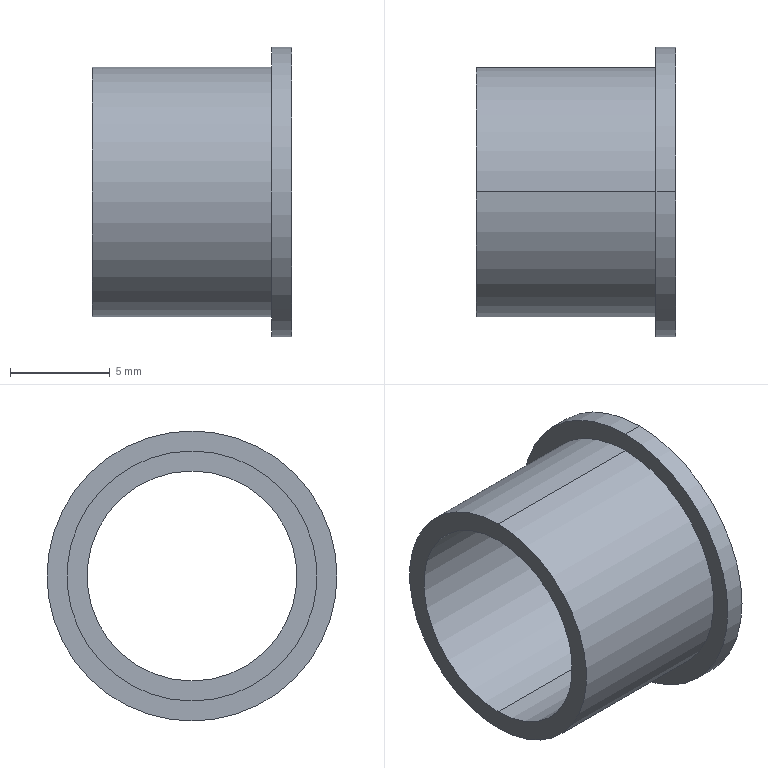Part | SolidWorks | features BaseBody 1 | 1 solid | 9 faces | box 10 x 14.5 x 14.5 mm | volume 403.695 mm3 | cylinder 6 | plane 3 | commonest cylinder face diameters 10.5 x2 12.5 x2 14.5 x2
STEP:
#1=CARTESIAN_POINT('',(6.037,-20.104,-31.5));
#2=VERTEX_POINT('',#1);
#3=CARTESIAN_POINT('',(6.037,-20.104,-46.));
#4=VERTEX_POINT('',#3);
#5=CARTESIAN_POINT('',(6.037,-20.104,-38.75));
#6=DIRECTION('',(-1.,0.,0.));
#7=DIRECTION('',(0.,0.,1.));
#8=AXIS2_PLACEMENT_3D('',#5,#6,#7);
#9=CIRCLE('',#8,7.25);
#10=EDGE_CURVE('',#2,#4,#9,.T.);
#11=ORIENTED_EDGE('',*,*,#10,.F.);
#12=CARTESIAN_POINT('',(7.037,-20.104,-31.5));
#13=VERTEX_POINT('',#12);
#14=CARTESIAN_POINT('',(6.037,-20.104,-31.5));
#15=DIRECTION('',(1.,0.,0.));
#16=VECTOR('',#15,1000.);
#17=LINE('',#14,#16);
#18=EDGE_CURVE('',#2,#13,#17,.T.);
#19=ORIENTED_EDGE('',*,*,#18,.T.);
#20=CARTESIAN_POINT('',(7.037,-20.104,-46.));
#21=VERTEX_POINT('',#20);
#22=CARTESIAN_POINT('',(7.037,-20.104,-38.75));
#23=DIRECTION('',(-1.,0.,0.));
#24=DIRECTION('',(0.,0.,1.));
#25=AXIS2_PLACEMENT_3D('',#22,#23,#24);
#26=CIRCLE('',#25,7.25);
#27=EDGE_CURVE('',#13,#21,#26,.T.);
#28=ORIENTED_EDGE('',*,*,#27,.T.);
#29=CARTESIAN_POINT('',(6.037,-20.104,-46.));
#30=DIRECTION('',(1.,0.,0.));
#31=VECTOR('',#30,1000.);
#32=LINE('',#29,#31);
#33=EDGE_CURVE('',#4,#21,#32,.T.);
#34=ORIENTED_EDGE('',*,*,#33,.F.);
#35=EDGE_LOOP('',(#11,#19,#28,#34));
#36=FACE_OUTER_BOUND('',#35,.T.);
#37=CARTESIAN_POINT('',(6.037,-20.104,-38.75));
#38=DIRECTION('',(1.,0.,0.));
#39=DIRECTION('',(0.,0.,-1.));
#40=AXIS2_PLACEMENT_3D('',#37,#38,#39);
#41=CYLINDRICAL_SURFACE('',#40,7.25);
#42=ADVANCED_FACE('',(#36),#41,.T.);
#43=CARTESIAN_POINT('',(-2.963,-20.104,-32.5));
#44=VERTEX_POINT('',#43);
#45=CARTESIAN_POINT('',(-2.963,-20.104,-45.));
#46=VERTEX_POINT('',#45);
#47=CARTESIAN_POINT('',(-2.963,-20.104,-38.75));
#48=DIRECTION('',(-1.,0.,0.));
#49=DIRECTION('',(0.,0.,1.));
#50=AXIS2_PLACEMENT_3D('',#47,#48,#49);
#51=CIRCLE('',#50,6.25);
#52=EDGE_CURVE('',#44,#46,#51,.T.);
#53=ORIENTED_EDGE('',*,*,#52,.F.);
#54=CARTESIAN_POINT('',(6.037,-20.104,-32.5));
#55=VERTEX_POINT('',#54);
#56=CARTESIAN_POINT('',(-2.963,-20.104,-32.5));
#57=DIRECTION('',(1.,0.,0.));
#58=VECTOR('',#57,1000.);
#59=LINE('',#56,#58);
#60=EDGE_CURVE('',#44,#55,#59,.T.);
#61=ORIENTED_EDGE('',*,*,#60,.T.);
#62=CARTESIAN_POINT('',(6.037,-20.104,-45.));
#63=VERTEX_POINT('',#62);
#64=CARTESIAN_POINT('',(6.037,-20.104,-38.75));
#65=DIRECTION('',(-1.,0.,0.));
#66=DIRECTION('',(0.,0.,1.));
#67=AXIS2_PLACEMENT_3D('',#64,#65,#66);
#68=CIRCLE('',#67,6.25);
#69=EDGE_CURVE('',#55,#63,#68,.T.);
#70=ORIENTED_EDGE('',*,*,#69,.T.);
#71=CARTESIAN_POINT('',(-2.963,-20.104,-45.));
#72=DIRECTION('',(1.,0.,0.));
#73=VECTOR('',#72,1000.);
#74=LINE('',#71,#73);
#75=EDGE_CURVE('',#46,#63,#74,.T.);
#76=ORIENTED_EDGE('',*,*,#75,.F.);
#77=EDGE_LOOP('',(#53,#61,#70,#76));
#78=FACE_OUTER_BOUND('',#77,.T.);
#79=CARTESIAN_POINT('',(-2.963,-20.104,-38.75));
#80=DIRECTION('',(1.,0.,0.));
#81=DIRECTION('',(0.,0.,-1.));
#82=AXIS2_PLACEMENT_3D('',#79,#80,#81);
#83=CYLINDRICAL_SURFACE('',#82,6.25);
#84=ADVANCED_FACE('',(#78),#83,.T.);
#85=CARTESIAN_POINT('',(7.037,-20.104,-44.));
#86=VERTEX_POINT('',#85);
#87=CARTESIAN_POINT('',(7.037,-20.104,-33.5));
#88=VERTEX_POINT('',#87);
#89=CARTESIAN_POINT('',(7.037,-20.104,-38.75));
#90=DIRECTION('',(-1.,0.,0.));
#91=DIRECTION('',(0.,0.,1.));
#92=AXIS2_PLACEMENT_3D('',#89,#90,#91);
#93=CIRCLE('',#92,5.25);
#94=EDGE_CURVE('',#86,#88,#93,.T.);
#95=ORIENTED_EDGE('',*,*,#94,.F.);
#96=CARTESIAN_POINT('',(-2.963,-20.104,-44.));
#97=VERTEX_POINT('',#96);
#98=CARTESIAN_POINT('',(7.037,-20.104,-44.));
#99=DIRECTION('',(-1.,0.,0.));
#100=VECTOR('',#99,1000.);
#101=LINE('',#98,#100);
#102=EDGE_CURVE('',#86,#97,#101,.T.);
#103=ORIENTED_EDGE('',*,*,#102,.T.);
#104=CARTESIAN_POINT('',(-2.963,-20.104,-33.5));
#105=VERTEX_POINT('',#104);
#106=CARTESIAN_POINT('',(-2.963,-20.104,-38.75));
#107=DIRECTION('',(-1.,0.,0.));
#108=DIRECTION('',(0.,0.,1.));
#109=AXIS2_PLACEMENT_3D('',#106,#107,#108);
#110=CIRCLE('',#109,5.25);
#111=EDGE_CURVE('',#97,#105,#110,.T.);
#112=ORIENTED_EDGE('',*,*,#111,.T.);
#113=CARTESIAN_POINT('',(7.037,-20.104,-33.5));
#114=DIRECTION('',(-1.,0.,0.));
#115=VECTOR('',#114,1000.);
#116=LINE('',#113,#115);
#117=EDGE_CURVE('',#88,#105,#116,.T.);
#118=ORIENTED_EDGE('',*,*,#117,.F.);
#119=EDGE_LOOP('',(#95,#103,#112,#118));
#120=FACE_OUTER_BOUND('',#119,.T.);
#121=CARTESIAN_POINT('',(7.037,-20.104,-38.75));
#122=DIRECTION('',(-1.,0.,0.));
#123=DIRECTION('',(0.,0.,1.));
#124=AXIS2_PLACEMENT_3D('',#121,#122,#123);
#125=CYLINDRICAL_SURFACE('',#124,5.25);
#126=ADVANCED_FACE('',(#120),#125,.F.);
#127=ORIENTED_EDGE('',*,*,#102,.F.);
#128=CARTESIAN_POINT('',(7.037,-20.104,-38.75));
#129=DIRECTION('',(-1.,0.,0.));
#130=DIRECTION('',(0.,0.,1.));
#131=AXIS2_PLACEMENT_3D('',#128,#129,#130);
#132=CIRCLE('',#131,5.25);
#133=EDGE_CURVE('',#88,#86,#132,.T.);
#134=ORIENTED_EDGE('',*,*,#133,.F.);
#135=ORIENTED_EDGE('',*,*,#117,.T.);
#136=CARTESIAN_POINT('',(-2.963,-20.104,-38.75));
#137=DIRECTION('',(-1.,0.,0.));
#138=DIRECTION('',(0.,0.,1.));
#139=AXIS2_PLACEMENT_3D('',#136,#137,#138);
#140=CIRCLE('',#139,5.25);
#141=EDGE_CURVE('',#105,#97,#140,.T.);
#142=ORIENTED_EDGE('',*,*,#141,.T.);
#143=EDGE_LOOP('',(#127,#134,#135,#142));
#144=FACE_OUTER_BOUND('',#143,.T.);
#145=CARTESIAN_POINT('',(7.037,-20.104,-38.75));
#146=DIRECTION('',(-1.,0.,0.));
#147=DIRECTION('',(0.,0.,1.));
#148=AXIS2_PLACEMENT_3D('',#145,#146,#147);
#149=CYLINDRICAL_SURFACE('',#148,5.25);
#150=ADVANCED_FACE('',(#144),#149,.F.);
#151=CARTESIAN_POINT('',(-2.963,-20.104,-38.75));
#152=DIRECTION('',(-1.,0.,0.));
#153=DIRECTION('',(0.,0.,1.));
#154=AXIS2_PLACEMENT_3D('',#151,#152,#153);
#155=CIRCLE('',#154,6.25);
#156=EDGE_CURVE('',#46,#44,#155,.T.);
#157=ORIENTED_EDGE('',*,*,#156,.T.);
#158=ORIENTED_EDGE('',*,*,#52,.T.);
#159=EDGE_LOOP('',(#157,#158));
#160=FACE_OUTER_BOUND('',#159,.T.);
#161=ORIENTED_EDGE('',*,*,#141,.F.);
#162=ORIENTED_EDGE('',*,*,#111,.F.);
#163=EDGE_LOOP('',(#161,#162));
#164=FACE_BOUND('',#163,.T.);
#165=CARTESIAN_POINT('',(-2.963,-20.104,-38.75));
#166=DIRECTION('',(-1.,0.,0.));
#167=DIRECTION('',(0.,1.,0.));
#168=AXIS2_PLACEMENT_3D('',#165,#166,#167);
#169=PLANE('',#168);
#170=ADVANCED_FACE('',(#160,#164),#169,.T.);
#171=ORIENTED_EDGE('',*,*,#60,.F.);
#172=ORIENTED_EDGE('',*,*,#156,.F.);
#173=ORIENTED_EDGE('',*,*,#75,.T.);
#174=CARTESIAN_POINT('',(6.037,-20.104,-38.75));
#175=DIRECTION('',(-1.,0.,0.));
#176=DIRECTION('',(0.,0.,1.));
#177=AXIS2_PLACEMENT_3D('',#174,#175,#176);
#178=CIRCLE('',#177,6.25);
#179=EDGE_CURVE('',#63,#55,#178,.T.);
#180=ORIENTED_EDGE('',*,*,#179,.T.);
#181=EDGE_LOOP('',(#171,#172,#173,#180));
#182=FACE_OUTER_BOUND('',#181,.T.);
#183=CARTESIAN_POINT('',(-2.963,-20.104,-38.75));
#184=DIRECTION('',(1.,0.,0.));
#185=DIRECTION('',(0.,0.,-1.));
#186=AXIS2_PLACEMENT_3D('',#183,#184,#185);
#187=CYLINDRICAL_SURFACE('',#186,6.25);
#188=ADVANCED_FACE('',(#182),#187,.T.);
#189=CARTESIAN_POINT('',(7.037,-20.104,-38.75));
#190=DIRECTION('',(-1.,0.,0.));
#191=DIRECTION('',(0.,0.,1.));
#192=AXIS2_PLACEMENT_3D('',#189,#190,#191);
#193=CIRCLE('',#192,7.25);
#194=EDGE_CURVE('',#21,#13,#193,.T.);
#195=ORIENTED_EDGE('',*,*,#194,.F.);
#196=ORIENTED_EDGE('',*,*,#27,.F.);
#197=EDGE_LOOP('',(#195,#196));
#198=FACE_OUTER_BOUND('',#197,.T.);
#199=ORIENTED_EDGE('',*,*,#133,.T.);
#200=ORIENTED_EDGE('',*,*,#94,.T.);
#201=EDGE_LOOP('',(#199,#200));
#202=FACE_BOUND('',#201,.T.);
#203=CARTESIAN_POINT('',(7.037,-20.104,-38.75));
#204=DIRECTION('',(-1.,0.,0.));
#205=DIRECTION('',(0.,1.,0.));
#206=AXIS2_PLACEMENT_3D('',#203,#204,#205);
#207=PLANE('',#206);
#208=ADVANCED_FACE('',(#198,#202),#207,.F.);
#209=CARTESIAN_POINT('',(6.037,-20.104,-38.75));
#210=DIRECTION('',(-1.,0.,0.));
#211=DIRECTION('',(0.,0.,1.));
#212=AXIS2_PLACEMENT_3D('',#209,#210,#211);
#213=CIRCLE('',#212,7.25);
#214=EDGE_CURVE('',#4,#2,#213,.T.);
#215=ORIENTED_EDGE('',*,*,#214,.T.);
#216=ORIENTED_EDGE('',*,*,#10,.T.);
#217=EDGE_LOOP('',(#215,#216));
#218=FACE_OUTER_BOUND('',#217,.T.);
#219=ORIENTED_EDGE('',*,*,#179,.F.);
#220=ORIENTED_EDGE('',*,*,#69,.F.);
#221=EDGE_LOOP('',(#219,#220));
#222=FACE_BOUND('',#221,.T.);
#223=CARTESIAN_POINT('',(6.037,-20.104,-38.75));
#224=DIRECTION('',(-1.,0.,0.));
#225=DIRECTION('',(0.,1.,0.));
#226=AXIS2_PLACEMENT_3D('',#223,#224,#225);
#227=PLANE('',#226);
#228=ADVANCED_FACE('',(#218,#222),#227,.T.);
#229=ORIENTED_EDGE('',*,*,#18,.F.);
#230=ORIENTED_EDGE('',*,*,#214,.F.);
#231=ORIENTED_EDGE('',*,*,#33,.T.);
#232=ORIENTED_EDGE('',*,*,#194,.T.);
#233=EDGE_LOOP('',(#229,#230,#231,#232));
#234=FACE_OUTER_BOUND('',#233,.T.);
#235=CARTESIAN_POINT('',(6.037,-20.104,-38.75));
#236=DIRECTION('',(1.,0.,0.));
#237=DIRECTION('',(0.,0.,-1.));
#238=AXIS2_PLACEMENT_3D('',#235,#236,#237);
#239=CYLINDRICAL_SURFACE('',#238,7.25);
#240=ADVANCED_FACE('',(#234),#239,.T.);
#241=CLOSED_SHELL('',(#42,#84,#126,#150,#170,#188,#208,#228,#240));
#242=MANIFOLD_SOLID_BREP('',#241);
#243=CARTESIAN_POINT('',(0.,0.,0.));
#244=DIRECTION('',(0.,0.,1.));
#245=DIRECTION('',(1.,0.,0.));
#246=AXIS2_PLACEMENT_3D('',#243,#244,#245);
#247=(LENGTH_UNIT()NAMED_UNIT(*)SI_UNIT(.MILLI.,.METRE.));
#248=UNCERTAINTY_MEASURE_WITH_UNIT(LENGTH_MEASURE(0.00001),#247,'','');
#249=(NAMED_UNIT(*)PLANE_ANGLE_UNIT()SI_UNIT($,.RADIAN.));
#250=(NAMED_UNIT(*)SI_UNIT($,.STERADIAN.)SOLID_ANGLE_UNIT());
#251=(GEOMETRIC_REPRESENTATION_CONTEXT(3)GLOBAL_UNCERTAINTY_ASSIGNED_CONTEXT((#248))GLOBAL_UNIT_ASSIGNED_CONTEXT((#247,#249,#250))REPRESENTATION_CONTEXT('',''));
#252=ADVANCED_BREP_SHAPE_REPRESENTATION('',(#242,#246),#251);